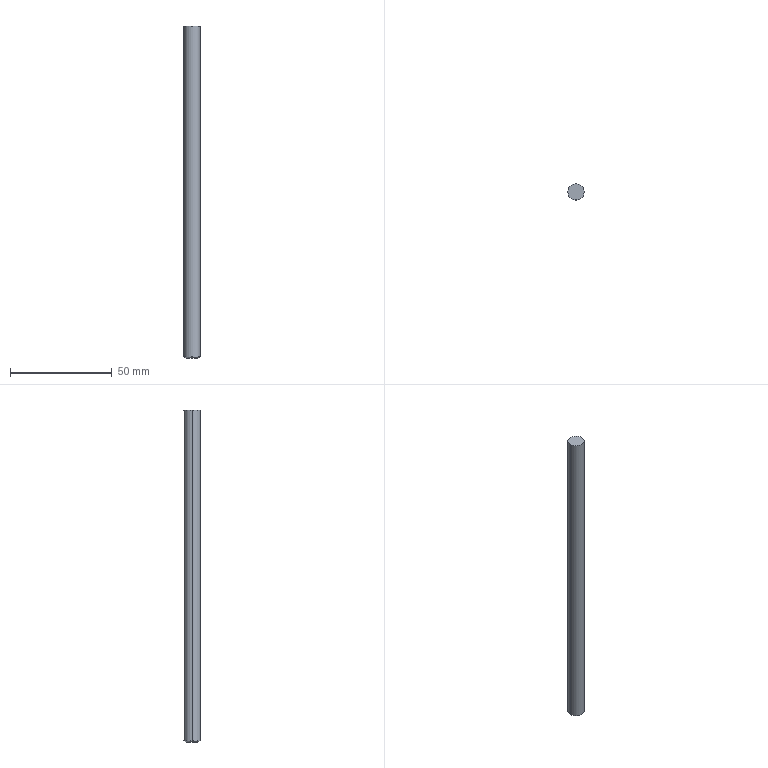Part | NX | features BREP 1, MOVE_FACE 1 | 1 solid | 6 faces | box 8 x 8 x 163 mm | volume 8186 mm3 | cone 2 | cylinder 2 | plane 2 | commonest cylinder face diameters 8 x2
STEP:
#1=CARTESIAN_POINT('',(2.917,0.,-1000.));
#2=VERTEX_POINT('',#1);
#3=CARTESIAN_POINT('',(-2.917,0.,-1000.));
#4=VERTEX_POINT('',#3);
#5=CARTESIAN_POINT('',(0.,0.,-1000.));
#6=DIRECTION('',(0.,0.,1.));
#7=DIRECTION('',(1.,0.,0.));
#8=AXIS2_PLACEMENT_3D('',#5,#6,#7);
#9=CIRCLE('',#8,2.917);
#10=EDGE_CURVE('',#2,#4,#9,.T.);
#11=ORIENTED_EDGE('',*,*,#10,.T.);
#12=CARTESIAN_POINT('',(-4.,0.,-999.375));
#13=VERTEX_POINT('',#12);
#14=CARTESIAN_POINT('',(-4.,0.,-999.375));
#15=DIRECTION('',(-0.866,0.,0.5));
#16=VECTOR('',#15,1000.);
#17=LINE('',#14,#16);
#18=EDGE_CURVE('',#4,#13,#17,.T.);
#19=ORIENTED_EDGE('',*,*,#18,.T.);
#20=CARTESIAN_POINT('',(4.,0.,-999.375));
#21=VERTEX_POINT('',#20);
#22=CARTESIAN_POINT('',(0.,0.,-999.375));
#23=DIRECTION('',(0.,0.,1.));
#24=DIRECTION('',(1.,0.,0.));
#25=AXIS2_PLACEMENT_3D('',#22,#23,#24);
#26=CIRCLE('',#25,4.);
#27=EDGE_CURVE('',#21,#13,#26,.T.);
#28=ORIENTED_EDGE('',*,*,#27,.F.);
#29=CARTESIAN_POINT('',(4.,0.,-999.375));
#30=DIRECTION('',(0.866,0.,0.5));
#31=VECTOR('',#30,1000.);
#32=LINE('',#29,#31);
#33=EDGE_CURVE('',#2,#21,#32,.T.);
#34=ORIENTED_EDGE('',*,*,#33,.F.);
#35=EDGE_LOOP('',(#11,#19,#28,#34));
#36=FACE_BOUND('',#35,.T.);
#37=CARTESIAN_POINT('',(0.,0.,-999.375));
#38=DIRECTION('',(0.,0.,1.));
#39=DIRECTION('',(-1.,0.,0.));
#40=AXIS2_PLACEMENT_3D('',#37,#38,#39);
#41=CONICAL_SURFACE('',#40,4.,1.047);
#42=ADVANCED_FACE('',(#36),#41,.T.);
#43=ORIENTED_EDGE('',*,*,#27,.T.);
#44=CARTESIAN_POINT('',(-4.,0.,-837.));
#45=VERTEX_POINT('',#44);
#46=CARTESIAN_POINT('',(-4.,0.,-1000.));
#47=DIRECTION('',(0.,0.,1.));
#48=VECTOR('',#47,1000.);
#49=LINE('',#46,#48);
#50=EDGE_CURVE('',#13,#45,#49,.T.);
#51=ORIENTED_EDGE('',*,*,#50,.T.);
#52=CARTESIAN_POINT('',(4.,0.,-837.));
#53=VERTEX_POINT('',#52);
#54=CARTESIAN_POINT('',(0.,0.,-837.));
#55=DIRECTION('',(0.,0.,1.));
#56=DIRECTION('',(1.,0.,0.));
#57=AXIS2_PLACEMENT_3D('',#54,#55,#56);
#58=CIRCLE('',#57,4.);
#59=EDGE_CURVE('',#53,#45,#58,.T.);
#60=ORIENTED_EDGE('',*,*,#59,.F.);
#61=CARTESIAN_POINT('',(4.,0.,-1000.));
#62=DIRECTION('',(0.,0.,1.));
#63=VECTOR('',#62,1000.);
#64=LINE('',#61,#63);
#65=EDGE_CURVE('',#21,#53,#64,.T.);
#66=ORIENTED_EDGE('',*,*,#65,.F.);
#67=EDGE_LOOP('',(#43,#51,#60,#66));
#68=FACE_BOUND('',#67,.T.);
#69=CARTESIAN_POINT('',(0.,0.,-1000.));
#70=DIRECTION('',(0.,0.,1.));
#71=DIRECTION('',(-1.,0.,0.));
#72=AXIS2_PLACEMENT_3D('',#69,#70,#71);
#73=CYLINDRICAL_SURFACE('',#72,4.);
#74=ADVANCED_FACE('',(#68),#73,.T.);
#75=ORIENTED_EDGE('',*,*,#50,.F.);
#76=CARTESIAN_POINT('',(0.,0.,-999.375));
#77=DIRECTION('',(0.,0.,1.));
#78=DIRECTION('',(1.,0.,0.));
#79=AXIS2_PLACEMENT_3D('',#76,#77,#78);
#80=CIRCLE('',#79,4.);
#81=EDGE_CURVE('',#13,#21,#80,.T.);
#82=ORIENTED_EDGE('',*,*,#81,.T.);
#83=ORIENTED_EDGE('',*,*,#65,.T.);
#84=CARTESIAN_POINT('',(0.,0.,-837.));
#85=DIRECTION('',(0.,0.,1.));
#86=DIRECTION('',(1.,0.,0.));
#87=AXIS2_PLACEMENT_3D('',#84,#85,#86);
#88=CIRCLE('',#87,4.);
#89=EDGE_CURVE('',#45,#53,#88,.T.);
#90=ORIENTED_EDGE('',*,*,#89,.F.);
#91=EDGE_LOOP('',(#75,#82,#83,#90));
#92=FACE_BOUND('',#91,.T.);
#93=CARTESIAN_POINT('',(0.,0.,-1000.));
#94=DIRECTION('',(0.,0.,1.));
#95=DIRECTION('',(-1.,0.,0.));
#96=AXIS2_PLACEMENT_3D('',#93,#94,#95);
#97=CYLINDRICAL_SURFACE('',#96,4.);
#98=ADVANCED_FACE('',(#92),#97,.T.);
#99=ORIENTED_EDGE('',*,*,#59,.T.);
#100=ORIENTED_EDGE('',*,*,#89,.T.);
#101=EDGE_LOOP('',(#99,#100));
#102=FACE_BOUND('',#101,.T.);
#103=CARTESIAN_POINT('',(0.,0.,-837.));
#104=DIRECTION('',(0.,0.,1.));
#105=DIRECTION('',(-1.,0.,0.));
#106=AXIS2_PLACEMENT_3D('',#103,#104,#105);
#107=PLANE('',#106);
#108=ADVANCED_FACE('',(#102),#107,.T.);
#109=ORIENTED_EDGE('',*,*,#18,.F.);
#110=CARTESIAN_POINT('',(0.,0.,-1000.));
#111=DIRECTION('',(0.,0.,1.));
#112=DIRECTION('',(1.,0.,0.));
#113=AXIS2_PLACEMENT_3D('',#110,#111,#112);
#114=CIRCLE('',#113,2.917);
#115=EDGE_CURVE('',#4,#2,#114,.T.);
#116=ORIENTED_EDGE('',*,*,#115,.T.);
#117=ORIENTED_EDGE('',*,*,#33,.T.);
#118=ORIENTED_EDGE('',*,*,#81,.F.);
#119=EDGE_LOOP('',(#109,#116,#117,#118));
#120=FACE_BOUND('',#119,.T.);
#121=CARTESIAN_POINT('',(0.,0.,-999.375));
#122=DIRECTION('',(0.,0.,1.));
#123=DIRECTION('',(-1.,0.,0.));
#124=AXIS2_PLACEMENT_3D('',#121,#122,#123);
#125=CONICAL_SURFACE('',#124,4.,1.047);
#126=ADVANCED_FACE('',(#120),#125,.T.);
#127=ORIENTED_EDGE('',*,*,#10,.F.);
#128=ORIENTED_EDGE('',*,*,#115,.F.);
#129=EDGE_LOOP('',(#127,#128));
#130=FACE_BOUND('',#129,.T.);
#131=CARTESIAN_POINT('',(0.,0.,-1000.));
#132=DIRECTION('',(0.,0.,1.));
#133=DIRECTION('',(-1.,0.,0.));
#134=AXIS2_PLACEMENT_3D('',#131,#132,#133);
#135=PLANE('',#134);
#136=ADVANCED_FACE('',(#130),#135,.F.);
#137=CLOSED_SHELL('',(#42,#74,#98,#108,#126,#136));
#138=MANIFOLD_SOLID_BREP('',#137);
#139=(LENGTH_UNIT()NAMED_UNIT(*)SI_UNIT(.MILLI.,.METRE.));
#140=UNCERTAINTY_MEASURE_WITH_UNIT(LENGTH_MEASURE(0.00001),#139,'','');
#141=(NAMED_UNIT(*)PLANE_ANGLE_UNIT()SI_UNIT($,.RADIAN.));
#142=(NAMED_UNIT(*)SI_UNIT($,.STERADIAN.)SOLID_ANGLE_UNIT());
#143=(GEOMETRIC_REPRESENTATION_CONTEXT(3)GLOBAL_UNCERTAINTY_ASSIGNED_CONTEXT((#140))GLOBAL_UNIT_ASSIGNED_CONTEXT((#139,#141,#142))REPRESENTATION_CONTEXT('',''));
#144=ADVANCED_BREP_SHAPE_REPRESENTATION('',(#138),#143);